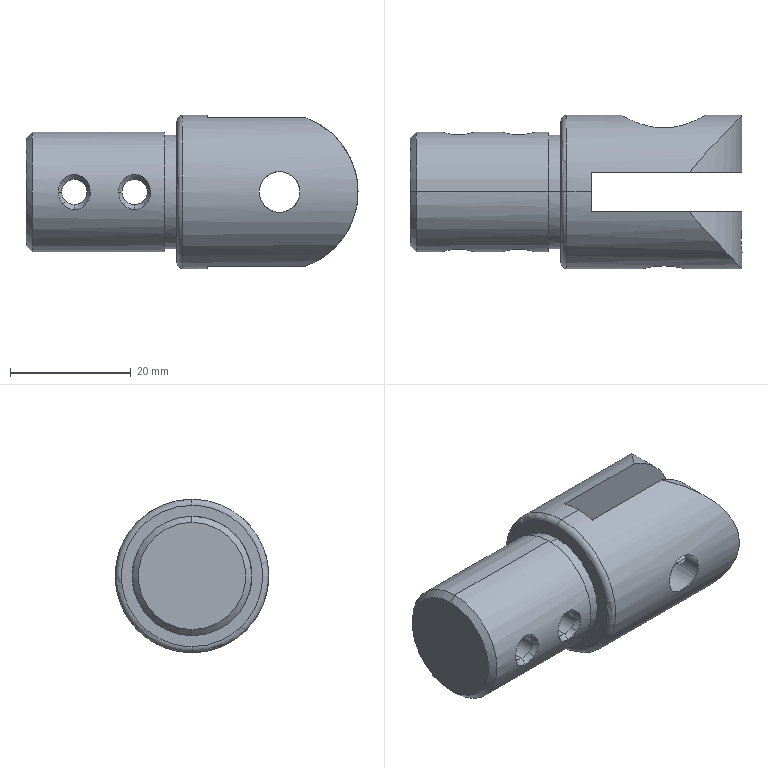Part | STEP file | 101000007783 | 1 solid | 76 faces | box 55 x 25.4 x 25.4 mm | volume 16233 mm3 | spline 45 | cylinder 20 | plane 7 | cone 2 | torus 2 | commonest cylinder face diameters 4.2 x4 6.75 x4 3.3 x2 14 x2 18.8 x2 19.8 x2